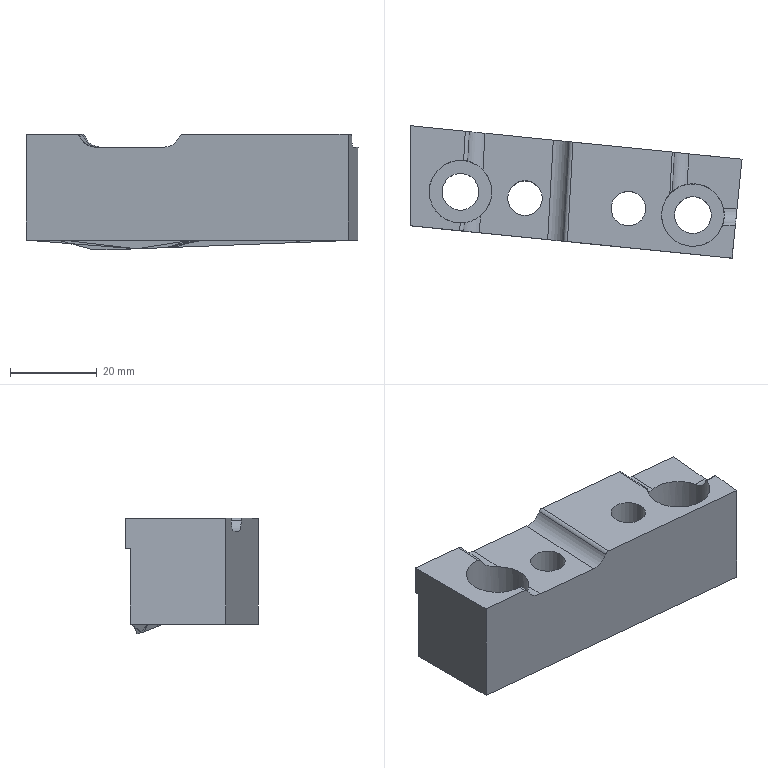Part | NX | features solid 2 | 1 solid | 29 faces | volume 31598 mm3 | cylinder 16 | plane 11 | spline 2 | commonest cylinder face diameters 2 x3 8 x3 1 x2 7 x2 8.001 x2 8.5 x2